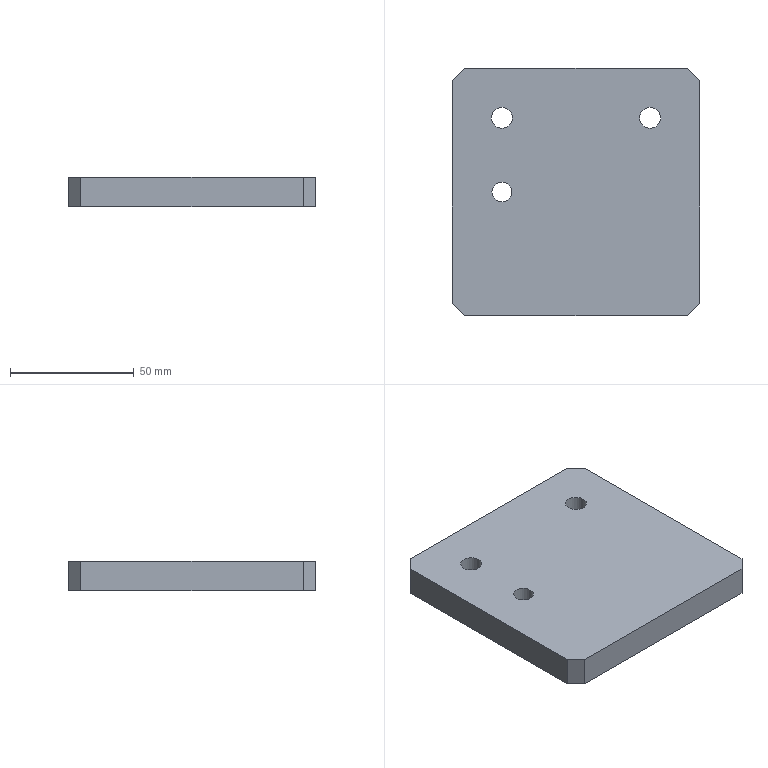Part | NX | features BREP 1 | 1 solid | 13 faces | box 100 x 100 x 12 mm | volume 117435 mm3 | plane 10 | cylinder 3 | commonest cylinder face diameters 8.5 x2 8 x1
STEP:
#1=CARTESIAN_POINT('',(50.,45.,3.));
#2=VERTEX_POINT('',#1);
#3=CARTESIAN_POINT('',(50.,-45.,3.));
#4=VERTEX_POINT('',#3);
#5=CARTESIAN_POINT('',(50.,50.,3.));
#6=DIRECTION('',(0.,-1.,0.));
#7=VECTOR('',#6,1000.);
#8=LINE('',#5,#7);
#9=EDGE_CURVE('',#2,#4,#8,.T.);
#10=ORIENTED_EDGE('',*,*,#9,.F.);
#11=CARTESIAN_POINT('',(50.,45.,15.));
#12=VERTEX_POINT('',#11);
#13=CARTESIAN_POINT('',(50.,45.,15.));
#14=DIRECTION('',(0.,0.,1.));
#15=VECTOR('',#14,1000.);
#16=LINE('',#13,#15);
#17=EDGE_CURVE('',#2,#12,#16,.T.);
#18=ORIENTED_EDGE('',*,*,#17,.T.);
#19=CARTESIAN_POINT('',(50.,-45.,15.));
#20=VERTEX_POINT('',#19);
#21=CARTESIAN_POINT('',(50.,50.,15.));
#22=DIRECTION('',(0.,1.,0.));
#23=VECTOR('',#22,1000.);
#24=LINE('',#21,#23);
#25=EDGE_CURVE('',#20,#12,#24,.T.);
#26=ORIENTED_EDGE('',*,*,#25,.F.);
#27=CARTESIAN_POINT('',(50.,-45.,15.));
#28=DIRECTION('',(0.,0.,-1.));
#29=VECTOR('',#28,1000.);
#30=LINE('',#27,#29);
#31=EDGE_CURVE('',#20,#4,#30,.T.);
#32=ORIENTED_EDGE('',*,*,#31,.T.);
#33=EDGE_LOOP('',(#10,#18,#26,#32));
#34=FACE_BOUND('',#33,.T.);
#35=CARTESIAN_POINT('',(50.,50.,15.));
#36=DIRECTION('',(-1.,0.,0.));
#37=DIRECTION('',(0.,0.,-1.));
#38=AXIS2_PLACEMENT_3D('',#35,#36,#37);
#39=PLANE('',#38);
#40=ADVANCED_FACE('',(#34),#39,.F.);
#41=CARTESIAN_POINT('',(45.,50.,3.));
#42=VERTEX_POINT('',#41);
#43=CARTESIAN_POINT('',(-45.,50.,3.));
#44=VERTEX_POINT('',#43);
#45=CARTESIAN_POINT('',(1330.,50.,3.));
#46=DIRECTION('',(-1.,0.,0.));
#47=VECTOR('',#46,1000.);
#48=LINE('',#45,#47);
#49=EDGE_CURVE('',#42,#44,#48,.T.);
#50=ORIENTED_EDGE('',*,*,#49,.T.);
#51=CARTESIAN_POINT('',(-45.,50.,15.));
#52=VERTEX_POINT('',#51);
#53=CARTESIAN_POINT('',(-45.,50.,15.));
#54=DIRECTION('',(0.,0.,1.));
#55=VECTOR('',#54,1000.);
#56=LINE('',#53,#55);
#57=EDGE_CURVE('',#44,#52,#56,.T.);
#58=ORIENTED_EDGE('',*,*,#57,.T.);
#59=CARTESIAN_POINT('',(45.,50.,15.));
#60=VERTEX_POINT('',#59);
#61=CARTESIAN_POINT('',(-50.,50.,15.));
#62=DIRECTION('',(-1.,0.,0.));
#63=VECTOR('',#62,1000.);
#64=LINE('',#61,#63);
#65=EDGE_CURVE('',#60,#52,#64,.T.);
#66=ORIENTED_EDGE('',*,*,#65,.F.);
#67=CARTESIAN_POINT('',(45.,50.,15.));
#68=DIRECTION('',(0.,0.,-1.));
#69=VECTOR('',#68,1000.);
#70=LINE('',#67,#69);
#71=EDGE_CURVE('',#60,#42,#70,.T.);
#72=ORIENTED_EDGE('',*,*,#71,.T.);
#73=EDGE_LOOP('',(#50,#58,#66,#72));
#74=FACE_BOUND('',#73,.T.);
#75=CARTESIAN_POINT('',(-50.,50.,15.));
#76=DIRECTION('',(0.,-1.,0.));
#77=DIRECTION('',(0.,0.,1.));
#78=AXIS2_PLACEMENT_3D('',#75,#76,#77);
#79=PLANE('',#78);
#80=ADVANCED_FACE('',(#74),#79,.F.);
#81=CARTESIAN_POINT('',(-50.,-45.,3.));
#82=VERTEX_POINT('',#81);
#83=CARTESIAN_POINT('',(-50.,45.,3.));
#84=VERTEX_POINT('',#83);
#85=CARTESIAN_POINT('',(-50.,50.,3.));
#86=DIRECTION('',(0.,1.,0.));
#87=VECTOR('',#86,1000.);
#88=LINE('',#85,#87);
#89=EDGE_CURVE('',#82,#84,#88,.T.);
#90=ORIENTED_EDGE('',*,*,#89,.F.);
#91=CARTESIAN_POINT('',(-50.,-45.,15.));
#92=VERTEX_POINT('',#91);
#93=CARTESIAN_POINT('',(-50.,-45.,15.));
#94=DIRECTION('',(0.,0.,1.));
#95=VECTOR('',#94,1000.);
#96=LINE('',#93,#95);
#97=EDGE_CURVE('',#82,#92,#96,.T.);
#98=ORIENTED_EDGE('',*,*,#97,.T.);
#99=CARTESIAN_POINT('',(-50.,45.,15.));
#100=VERTEX_POINT('',#99);
#101=CARTESIAN_POINT('',(-50.,50.,15.));
#102=DIRECTION('',(0.,-1.,0.));
#103=VECTOR('',#102,1000.);
#104=LINE('',#101,#103);
#105=EDGE_CURVE('',#100,#92,#104,.T.);
#106=ORIENTED_EDGE('',*,*,#105,.F.);
#107=CARTESIAN_POINT('',(-50.,45.,15.));
#108=DIRECTION('',(0.,0.,-1.));
#109=VECTOR('',#108,1000.);
#110=LINE('',#107,#109);
#111=EDGE_CURVE('',#100,#84,#110,.T.);
#112=ORIENTED_EDGE('',*,*,#111,.T.);
#113=EDGE_LOOP('',(#90,#98,#106,#112));
#114=FACE_BOUND('',#113,.T.);
#115=CARTESIAN_POINT('',(-50.,50.,15.));
#116=DIRECTION('',(1.,0.,0.));
#117=DIRECTION('',(0.,-1.,0.));
#118=AXIS2_PLACEMENT_3D('',#115,#116,#117);
#119=PLANE('',#118);
#120=ADVANCED_FACE('',(#114),#119,.F.);
#121=CARTESIAN_POINT('',(45.,-50.,3.));
#122=VERTEX_POINT('',#121);
#123=CARTESIAN_POINT('',(-45.,-50.,3.));
#124=VERTEX_POINT('',#123);
#125=CARTESIAN_POINT('',(-50.,-50.,3.));
#126=DIRECTION('',(-1.,0.,0.));
#127=VECTOR('',#126,1000.);
#128=LINE('',#125,#127);
#129=EDGE_CURVE('',#122,#124,#128,.T.);
#130=ORIENTED_EDGE('',*,*,#129,.F.);
#131=CARTESIAN_POINT('',(45.,-50.,15.));
#132=VERTEX_POINT('',#131);
#133=CARTESIAN_POINT('',(45.,-50.,15.));
#134=DIRECTION('',(0.,0.,1.));
#135=VECTOR('',#134,1000.);
#136=LINE('',#133,#135);
#137=EDGE_CURVE('',#122,#132,#136,.T.);
#138=ORIENTED_EDGE('',*,*,#137,.T.);
#139=CARTESIAN_POINT('',(-45.,-50.,15.));
#140=VERTEX_POINT('',#139);
#141=CARTESIAN_POINT('',(-50.,-50.,15.));
#142=DIRECTION('',(1.,0.,0.));
#143=VECTOR('',#142,1000.);
#144=LINE('',#141,#143);
#145=EDGE_CURVE('',#140,#132,#144,.T.);
#146=ORIENTED_EDGE('',*,*,#145,.F.);
#147=CARTESIAN_POINT('',(-45.,-50.,15.));
#148=DIRECTION('',(0.,0.,-1.));
#149=VECTOR('',#148,1000.);
#150=LINE('',#147,#149);
#151=EDGE_CURVE('',#140,#124,#150,.T.);
#152=ORIENTED_EDGE('',*,*,#151,.T.);
#153=EDGE_LOOP('',(#130,#138,#146,#152));
#154=FACE_BOUND('',#153,.T.);
#155=CARTESIAN_POINT('',(-50.,-50.,15.));
#156=DIRECTION('',(0.,1.,0.));
#157=DIRECTION('',(0.,0.,-1.));
#158=AXIS2_PLACEMENT_3D('',#155,#156,#157);
#159=PLANE('',#158);
#160=ADVANCED_FACE('',(#154),#159,.F.);
#161=ORIENTED_EDGE('',*,*,#97,.F.);
#162=CARTESIAN_POINT('',(-45.,-50.,3.));
#163=DIRECTION('',(0.7071,-0.7071,0.));
#164=VECTOR('',#163,1000.);
#165=LINE('',#162,#164);
#166=EDGE_CURVE('',#82,#124,#165,.T.);
#167=ORIENTED_EDGE('',*,*,#166,.T.);
#168=ORIENTED_EDGE('',*,*,#151,.F.);
#169=CARTESIAN_POINT('',(-47.5,-47.5,15.));
#170=DIRECTION('',(0.7071,-0.7071,0.));
#171=VECTOR('',#170,1000.);
#172=LINE('',#169,#171);
#173=EDGE_CURVE('',#92,#140,#172,.T.);
#174=ORIENTED_EDGE('',*,*,#173,.F.);
#175=EDGE_LOOP('',(#161,#167,#168,#174));
#176=FACE_BOUND('',#175,.T.);
#177=CARTESIAN_POINT('',(-45.,-50.,15.));
#178=DIRECTION('',(0.7071,0.7071,0.));
#179=DIRECTION('',(0.,0.,1.));
#180=AXIS2_PLACEMENT_3D('',#177,#178,#179);
#181=PLANE('',#180);
#182=ADVANCED_FACE('',(#176),#181,.F.);
#183=ORIENTED_EDGE('',*,*,#137,.F.);
#184=CARTESIAN_POINT('',(50.,-45.,3.));
#185=DIRECTION('',(0.7071,0.7071,0.));
#186=VECTOR('',#185,1000.);
#187=LINE('',#184,#186);
#188=EDGE_CURVE('',#122,#4,#187,.T.);
#189=ORIENTED_EDGE('',*,*,#188,.T.);
#190=ORIENTED_EDGE('',*,*,#31,.F.);
#191=CARTESIAN_POINT('',(47.5,-47.5,15.));
#192=DIRECTION('',(0.7071,0.7071,0.));
#193=VECTOR('',#192,1000.);
#194=LINE('',#191,#193);
#195=EDGE_CURVE('',#132,#20,#194,.T.);
#196=ORIENTED_EDGE('',*,*,#195,.F.);
#197=EDGE_LOOP('',(#183,#189,#190,#196));
#198=FACE_BOUND('',#197,.T.);
#199=CARTESIAN_POINT('',(50.,-45.,15.));
#200=DIRECTION('',(-0.7071,0.7071,0.));
#201=DIRECTION('',(0.,0.,1.));
#202=AXIS2_PLACEMENT_3D('',#199,#200,#201);
#203=PLANE('',#202);
#204=ADVANCED_FACE('',(#198),#203,.F.);
#205=ORIENTED_EDGE('',*,*,#17,.F.);
#206=CARTESIAN_POINT('',(45.,50.,3.));
#207=DIRECTION('',(-0.7071,0.7071,0.));
#208=VECTOR('',#207,1000.);
#209=LINE('',#206,#208);
#210=EDGE_CURVE('',#2,#42,#209,.T.);
#211=ORIENTED_EDGE('',*,*,#210,.T.);
#212=ORIENTED_EDGE('',*,*,#71,.F.);
#213=CARTESIAN_POINT('',(47.5,47.5,15.));
#214=DIRECTION('',(-0.7071,0.7071,0.));
#215=VECTOR('',#214,1000.);
#216=LINE('',#213,#215);
#217=EDGE_CURVE('',#12,#60,#216,.T.);
#218=ORIENTED_EDGE('',*,*,#217,.F.);
#219=EDGE_LOOP('',(#205,#211,#212,#218));
#220=FACE_BOUND('',#219,.T.);
#221=CARTESIAN_POINT('',(45.,50.,15.));
#222=DIRECTION('',(-0.7071,-0.7071,0.));
#223=DIRECTION('',(0.,0.,1.));
#224=AXIS2_PLACEMENT_3D('',#221,#222,#223);
#225=PLANE('',#224);
#226=ADVANCED_FACE('',(#220),#225,.F.);
#227=ORIENTED_EDGE('',*,*,#57,.F.);
#228=CARTESIAN_POINT('',(-50.,45.,3.));
#229=DIRECTION('',(-0.7071,-0.7071,0.));
#230=VECTOR('',#229,1000.);
#231=LINE('',#228,#230);
#232=EDGE_CURVE('',#44,#84,#231,.T.);
#233=ORIENTED_EDGE('',*,*,#232,.T.);
#234=ORIENTED_EDGE('',*,*,#111,.F.);
#235=CARTESIAN_POINT('',(-47.5,47.5,15.));
#236=DIRECTION('',(-0.7071,-0.7071,0.));
#237=VECTOR('',#236,1000.);
#238=LINE('',#235,#237);
#239=EDGE_CURVE('',#52,#100,#238,.T.);
#240=ORIENTED_EDGE('',*,*,#239,.F.);
#241=EDGE_LOOP('',(#227,#233,#234,#240));
#242=FACE_BOUND('',#241,.T.);
#243=CARTESIAN_POINT('',(-50.,45.,15.));
#244=DIRECTION('',(0.7071,-0.7071,0.));
#245=DIRECTION('',(0.,0.,1.));
#246=AXIS2_PLACEMENT_3D('',#243,#244,#245);
#247=PLANE('',#246);
#248=ADVANCED_FACE('',(#242),#247,.F.);
#249=CARTESIAN_POINT('',(-25.75,30.,15.));
#250=VERTEX_POINT('',#249);
#251=CARTESIAN_POINT('',(-30.,30.,15.));
#252=DIRECTION('',(0.,0.,1.));
#253=DIRECTION('',(1.,0.,0.));
#254=AXIS2_PLACEMENT_3D('',#251,#252,#253);
#255=CIRCLE('',#254,4.25);
#256=EDGE_CURVE('',#250,#250,#255,.T.);
#257=ORIENTED_EDGE('',*,*,#256,.F.);
#258=EDGE_LOOP('',(#257));
#259=FACE_BOUND('',#258,.T.);
#260=CARTESIAN_POINT('',(34.25,30.,15.));
#261=VERTEX_POINT('',#260);
#262=CARTESIAN_POINT('',(30.,30.,15.));
#263=DIRECTION('',(0.,0.,1.));
#264=DIRECTION('',(1.,0.,0.));
#265=AXIS2_PLACEMENT_3D('',#262,#263,#264);
#266=CIRCLE('',#265,4.25);
#267=EDGE_CURVE('',#261,#261,#266,.T.);
#268=ORIENTED_EDGE('',*,*,#267,.F.);
#269=EDGE_LOOP('',(#268));
#270=FACE_BOUND('',#269,.T.);
#271=CARTESIAN_POINT('',(-26.,0.,15.));
#272=VERTEX_POINT('',#271);
#273=CARTESIAN_POINT('',(-30.,0.,15.));
#274=DIRECTION('',(0.,0.,1.));
#275=DIRECTION('',(1.,0.,0.));
#276=AXIS2_PLACEMENT_3D('',#273,#274,#275);
#277=CIRCLE('',#276,4.);
#278=EDGE_CURVE('',#272,#272,#277,.T.);
#279=ORIENTED_EDGE('',*,*,#278,.F.);
#280=EDGE_LOOP('',(#279));
#281=FACE_BOUND('',#280,.T.);
#282=ORIENTED_EDGE('',*,*,#105,.T.);
#283=ORIENTED_EDGE('',*,*,#173,.T.);
#284=ORIENTED_EDGE('',*,*,#145,.T.);
#285=ORIENTED_EDGE('',*,*,#195,.T.);
#286=ORIENTED_EDGE('',*,*,#25,.T.);
#287=ORIENTED_EDGE('',*,*,#217,.T.);
#288=ORIENTED_EDGE('',*,*,#65,.T.);
#289=ORIENTED_EDGE('',*,*,#239,.T.);
#290=EDGE_LOOP('',(#282,#283,#284,#285,#286,#287,#288,#289));
#291=FACE_BOUND('',#290,.T.);
#292=CARTESIAN_POINT('',(0.,0.,15.));
#293=DIRECTION('',(0.,0.,1.));
#294=DIRECTION('',(-1.,0.,0.));
#295=AXIS2_PLACEMENT_3D('',#292,#293,#294);
#296=PLANE('',#295);
#297=ADVANCED_FACE('',(#259,#270,#281,#291),#296,.T.);
#298=CARTESIAN_POINT('',(-34.25,30.,3.));
#299=VERTEX_POINT('',#298);
#300=CARTESIAN_POINT('',(-30.,30.,3.));
#301=DIRECTION('',(0.,0.,-1.));
#302=DIRECTION('',(-1.,0.,0.));
#303=AXIS2_PLACEMENT_3D('',#300,#301,#302);
#304=CIRCLE('',#303,4.25);
#305=EDGE_CURVE('',#299,#299,#304,.T.);
#306=ORIENTED_EDGE('',*,*,#305,.F.);
#307=EDGE_LOOP('',(#306));
#308=FACE_BOUND('',#307,.T.);
#309=CARTESIAN_POINT('',(25.75,30.,3.));
#310=VERTEX_POINT('',#309);
#311=CARTESIAN_POINT('',(30.,30.,3.));
#312=DIRECTION('',(0.,0.,-1.));
#313=DIRECTION('',(-1.,0.,0.));
#314=AXIS2_PLACEMENT_3D('',#311,#312,#313);
#315=CIRCLE('',#314,4.25);
#316=EDGE_CURVE('',#310,#310,#315,.T.);
#317=ORIENTED_EDGE('',*,*,#316,.F.);
#318=EDGE_LOOP('',(#317));
#319=FACE_BOUND('',#318,.T.);
#320=CARTESIAN_POINT('',(-34.,0.,3.));
#321=VERTEX_POINT('',#320);
#322=CARTESIAN_POINT('',(-30.,0.,3.));
#323=DIRECTION('',(0.,0.,-1.));
#324=DIRECTION('',(-1.,0.,0.));
#325=AXIS2_PLACEMENT_3D('',#322,#323,#324);
#326=CIRCLE('',#325,4.);
#327=EDGE_CURVE('',#321,#321,#326,.T.);
#328=ORIENTED_EDGE('',*,*,#327,.F.);
#329=EDGE_LOOP('',(#328));
#330=FACE_BOUND('',#329,.T.);
#331=ORIENTED_EDGE('',*,*,#9,.T.);
#332=ORIENTED_EDGE('',*,*,#188,.F.);
#333=ORIENTED_EDGE('',*,*,#129,.T.);
#334=ORIENTED_EDGE('',*,*,#166,.F.);
#335=ORIENTED_EDGE('',*,*,#89,.T.);
#336=ORIENTED_EDGE('',*,*,#232,.F.);
#337=ORIENTED_EDGE('',*,*,#49,.F.);
#338=ORIENTED_EDGE('',*,*,#210,.F.);
#339=EDGE_LOOP('',(#331,#332,#333,#334,#335,#336,#337,#338));
#340=FACE_BOUND('',#339,.T.);
#341=CARTESIAN_POINT('',(380.,-300.,3.));
#342=DIRECTION('',(0.,0.,-1.));
#343=DIRECTION('',(1.,0.,0.));
#344=AXIS2_PLACEMENT_3D('',#341,#342,#343);
#345=PLANE('',#344);
#346=ADVANCED_FACE('',(#308,#319,#330,#340),#345,.T.);
#347=ORIENTED_EDGE('',*,*,#278,.T.);
#348=EDGE_LOOP('',(#347));
#349=FACE_BOUND('',#348,.T.);
#350=ORIENTED_EDGE('',*,*,#327,.T.);
#351=EDGE_LOOP('',(#350));
#352=FACE_BOUND('',#351,.T.);
#353=CARTESIAN_POINT('',(-30.,0.,3.));
#354=DIRECTION('',(0.,0.,-1.));
#355=DIRECTION('',(1.,0.,0.));
#356=AXIS2_PLACEMENT_3D('',#353,#354,#355);
#357=CYLINDRICAL_SURFACE('',#356,4.);
#358=ADVANCED_FACE('',(#349,#352),#357,.F.);
#359=ORIENTED_EDGE('',*,*,#267,.T.);
#360=EDGE_LOOP('',(#359));
#361=FACE_BOUND('',#360,.T.);
#362=ORIENTED_EDGE('',*,*,#316,.T.);
#363=EDGE_LOOP('',(#362));
#364=FACE_BOUND('',#363,.T.);
#365=CARTESIAN_POINT('',(30.,30.,3.));
#366=DIRECTION('',(0.,0.,-1.));
#367=DIRECTION('',(1.,0.,0.));
#368=AXIS2_PLACEMENT_3D('',#365,#366,#367);
#369=CYLINDRICAL_SURFACE('',#368,4.25);
#370=ADVANCED_FACE('',(#361,#364),#369,.F.);
#371=ORIENTED_EDGE('',*,*,#256,.T.);
#372=EDGE_LOOP('',(#371));
#373=FACE_BOUND('',#372,.T.);
#374=ORIENTED_EDGE('',*,*,#305,.T.);
#375=EDGE_LOOP('',(#374));
#376=FACE_BOUND('',#375,.T.);
#377=CARTESIAN_POINT('',(-30.,30.,3.));
#378=DIRECTION('',(0.,0.,-1.));
#379=DIRECTION('',(1.,0.,0.));
#380=AXIS2_PLACEMENT_3D('',#377,#378,#379);
#381=CYLINDRICAL_SURFACE('',#380,4.25);
#382=ADVANCED_FACE('',(#373,#376),#381,.F.);
#383=CLOSED_SHELL('',(#40,#80,#120,#160,#182,#204,#226,#248,#297,#346,#358,#370,#382));
#384=MANIFOLD_SOLID_BREP('',#383);
#385=(LENGTH_UNIT()NAMED_UNIT(*)SI_UNIT(.MILLI.,.METRE.));
#386=UNCERTAINTY_MEASURE_WITH_UNIT(LENGTH_MEASURE(0.00001),#385,'','');
#387=(NAMED_UNIT(*)PLANE_ANGLE_UNIT()SI_UNIT($,.RADIAN.));
#388=(NAMED_UNIT(*)SI_UNIT($,.STERADIAN.)SOLID_ANGLE_UNIT());
#389=(GEOMETRIC_REPRESENTATION_CONTEXT(3)GLOBAL_UNCERTAINTY_ASSIGNED_CONTEXT((#386))GLOBAL_UNIT_ASSIGNED_CONTEXT((#385,#387,#388))REPRESENTATION_CONTEXT('',''));
#390=ADVANCED_BREP_SHAPE_REPRESENTATION('',(#384),#389);